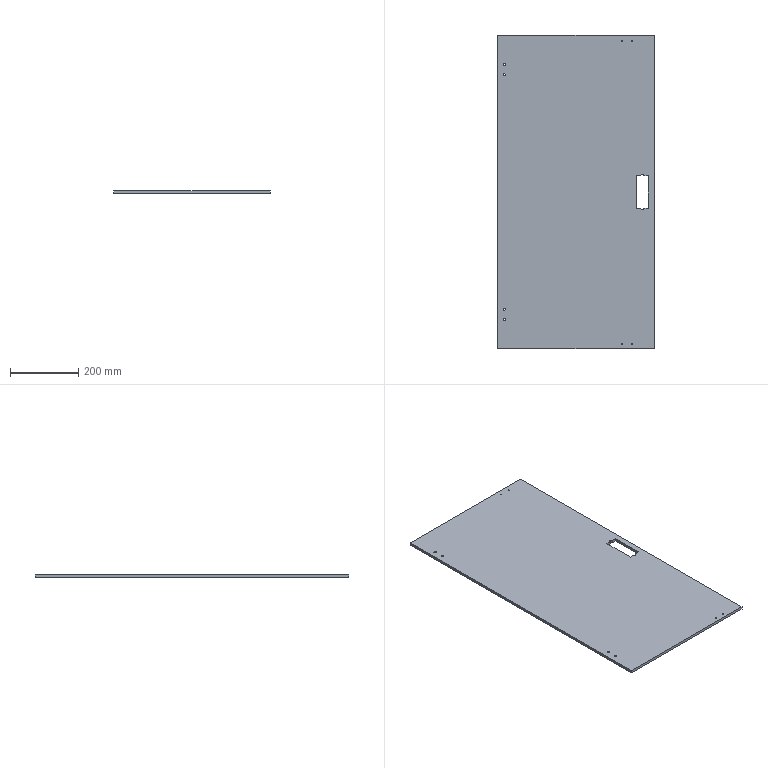Part | STEP file | Left door panel_PN_0002 | 1 solid | 30 faces | box 458.5 x 917 x 8 mm | volume 3334170 mm3 | cylinder 18 | plane 12 | commonest cylinder face diameters 3.3 x8 6.5 x8 8 x2
STEP:
#1=CARTESIAN_POINT('',(-207.,373.5,-4.));
#2=VERTEX_POINT('',#1);
#3=CARTESIAN_POINT('',(-213.5,373.5,-4.));
#4=VERTEX_POINT('',#3);
#5=CARTESIAN_POINT('',(-210.25,373.5,-4.));
#6=DIRECTION('',(0.,0.,-1.));
#7=DIRECTION('',(1.,0.,0.));
#8=AXIS2_PLACEMENT_3D('',#5,#6,#7);
#9=CIRCLE('',#8,3.25);
#10=EDGE_CURVE('',#2,#4,#9,.T.);
#11=ORIENTED_EDGE('',*,*,#10,.T.);
#12=CARTESIAN_POINT('',(-213.5,373.5,4.));
#13=VERTEX_POINT('',#12);
#14=CARTESIAN_POINT('',(-213.5,373.5,-4.));
#15=DIRECTION('',(0.,0.,1.));
#16=VECTOR('',#15,1000.);
#17=LINE('',#14,#16);
#18=EDGE_CURVE('',#4,#13,#17,.T.);
#19=ORIENTED_EDGE('',*,*,#18,.T.);
#20=CARTESIAN_POINT('',(-207.,373.5,4.));
#21=VERTEX_POINT('',#20);
#22=CARTESIAN_POINT('',(-210.25,373.5,4.));
#23=DIRECTION('',(0.,0.,-1.));
#24=DIRECTION('',(1.,0.,0.));
#25=AXIS2_PLACEMENT_3D('',#22,#23,#24);
#26=CIRCLE('',#25,3.25);
#27=EDGE_CURVE('',#21,#13,#26,.T.);
#28=ORIENTED_EDGE('',*,*,#27,.F.);
#29=CARTESIAN_POINT('',(-207.,373.5,-4.));
#30=DIRECTION('',(0.,0.,1.));
#31=VECTOR('',#30,1000.);
#32=LINE('',#29,#31);
#33=EDGE_CURVE('',#2,#21,#32,.T.);
#34=ORIENTED_EDGE('',*,*,#33,.F.);
#35=EDGE_LOOP('',(#11,#19,#28,#34));
#36=FACE_OUTER_BOUND('',#35,.T.);
#37=CARTESIAN_POINT('',(-210.25,373.5,-4.));
#38=DIRECTION('',(0.,0.,1.));
#39=DIRECTION('',(1.,0.,0.));
#40=AXIS2_PLACEMENT_3D('',#37,#38,#39);
#41=CYLINDRICAL_SURFACE('',#40,3.25);
#42=ADVANCED_FACE('',(#36),#41,.F.);
#43=CARTESIAN_POINT('',(-207.,343.5,-4.));
#44=VERTEX_POINT('',#43);
#45=CARTESIAN_POINT('',(-213.5,343.5,-4.));
#46=VERTEX_POINT('',#45);
#47=CARTESIAN_POINT('',(-210.25,343.5,-4.));
#48=DIRECTION('',(0.,0.,-1.));
#49=DIRECTION('',(1.,0.,0.));
#50=AXIS2_PLACEMENT_3D('',#47,#48,#49);
#51=CIRCLE('',#50,3.25);
#52=EDGE_CURVE('',#44,#46,#51,.T.);
#53=ORIENTED_EDGE('',*,*,#52,.T.);
#54=CARTESIAN_POINT('',(-213.5,343.5,4.));
#55=VERTEX_POINT('',#54);
#56=CARTESIAN_POINT('',(-213.5,343.5,-4.));
#57=DIRECTION('',(0.,0.,1.));
#58=VECTOR('',#57,1000.);
#59=LINE('',#56,#58);
#60=EDGE_CURVE('',#46,#55,#59,.T.);
#61=ORIENTED_EDGE('',*,*,#60,.T.);
#62=CARTESIAN_POINT('',(-207.,343.5,4.));
#63=VERTEX_POINT('',#62);
#64=CARTESIAN_POINT('',(-210.25,343.5,4.));
#65=DIRECTION('',(0.,0.,-1.));
#66=DIRECTION('',(1.,0.,0.));
#67=AXIS2_PLACEMENT_3D('',#64,#65,#66);
#68=CIRCLE('',#67,3.25);
#69=EDGE_CURVE('',#63,#55,#68,.T.);
#70=ORIENTED_EDGE('',*,*,#69,.F.);
#71=CARTESIAN_POINT('',(-207.,343.5,-4.));
#72=DIRECTION('',(0.,0.,1.));
#73=VECTOR('',#72,1000.);
#74=LINE('',#71,#73);
#75=EDGE_CURVE('',#44,#63,#74,.T.);
#76=ORIENTED_EDGE('',*,*,#75,.F.);
#77=EDGE_LOOP('',(#53,#61,#70,#76));
#78=FACE_OUTER_BOUND('',#77,.T.);
#79=CARTESIAN_POINT('',(-210.25,343.5,-4.));
#80=DIRECTION('',(0.,0.,1.));
#81=DIRECTION('',(1.,0.,0.));
#82=AXIS2_PLACEMENT_3D('',#79,#80,#81);
#83=CYLINDRICAL_SURFACE('',#82,3.25);
#84=ADVANCED_FACE('',(#78),#83,.F.);
#85=CARTESIAN_POINT('',(-207.,-343.5,-4.));
#86=VERTEX_POINT('',#85);
#87=CARTESIAN_POINT('',(-213.5,-343.5,-4.));
#88=VERTEX_POINT('',#87);
#89=CARTESIAN_POINT('',(-210.25,-343.5,-4.));
#90=DIRECTION('',(0.,0.,-1.));
#91=DIRECTION('',(1.,0.,0.));
#92=AXIS2_PLACEMENT_3D('',#89,#90,#91);
#93=CIRCLE('',#92,3.25);
#94=EDGE_CURVE('',#86,#88,#93,.T.);
#95=ORIENTED_EDGE('',*,*,#94,.T.);
#96=CARTESIAN_POINT('',(-213.5,-343.5,4.));
#97=VERTEX_POINT('',#96);
#98=CARTESIAN_POINT('',(-213.5,-343.5,-4.));
#99=DIRECTION('',(0.,0.,1.));
#100=VECTOR('',#99,1000.);
#101=LINE('',#98,#100);
#102=EDGE_CURVE('',#88,#97,#101,.T.);
#103=ORIENTED_EDGE('',*,*,#102,.T.);
#104=CARTESIAN_POINT('',(-207.,-343.5,4.));
#105=VERTEX_POINT('',#104);
#106=CARTESIAN_POINT('',(-210.25,-343.5,4.));
#107=DIRECTION('',(0.,0.,-1.));
#108=DIRECTION('',(1.,0.,0.));
#109=AXIS2_PLACEMENT_3D('',#106,#107,#108);
#110=CIRCLE('',#109,3.25);
#111=EDGE_CURVE('',#105,#97,#110,.T.);
#112=ORIENTED_EDGE('',*,*,#111,.F.);
#113=CARTESIAN_POINT('',(-207.,-343.5,-4.));
#114=DIRECTION('',(0.,0.,1.));
#115=VECTOR('',#114,1000.);
#116=LINE('',#113,#115);
#117=EDGE_CURVE('',#86,#105,#116,.T.);
#118=ORIENTED_EDGE('',*,*,#117,.F.);
#119=EDGE_LOOP('',(#95,#103,#112,#118));
#120=FACE_OUTER_BOUND('',#119,.T.);
#121=CARTESIAN_POINT('',(-210.25,-343.5,-4.));
#122=DIRECTION('',(0.,0.,1.));
#123=DIRECTION('',(1.,0.,0.));
#124=AXIS2_PLACEMENT_3D('',#121,#122,#123);
#125=CYLINDRICAL_SURFACE('',#124,3.25);
#126=ADVANCED_FACE('',(#120),#125,.F.);
#127=CARTESIAN_POINT('',(-207.,-373.5,-4.));
#128=VERTEX_POINT('',#127);
#129=CARTESIAN_POINT('',(-213.5,-373.5,-4.));
#130=VERTEX_POINT('',#129);
#131=CARTESIAN_POINT('',(-210.25,-373.5,-4.));
#132=DIRECTION('',(0.,0.,-1.));
#133=DIRECTION('',(1.,0.,0.));
#134=AXIS2_PLACEMENT_3D('',#131,#132,#133);
#135=CIRCLE('',#134,3.25);
#136=EDGE_CURVE('',#128,#130,#135,.T.);
#137=ORIENTED_EDGE('',*,*,#136,.T.);
#138=CARTESIAN_POINT('',(-213.5,-373.5,4.));
#139=VERTEX_POINT('',#138);
#140=CARTESIAN_POINT('',(-213.5,-373.5,-4.));
#141=DIRECTION('',(0.,0.,1.));
#142=VECTOR('',#141,1000.);
#143=LINE('',#140,#142);
#144=EDGE_CURVE('',#130,#139,#143,.T.);
#145=ORIENTED_EDGE('',*,*,#144,.T.);
#146=CARTESIAN_POINT('',(-207.,-373.5,4.));
#147=VERTEX_POINT('',#146);
#148=CARTESIAN_POINT('',(-210.25,-373.5,4.));
#149=DIRECTION('',(0.,0.,-1.));
#150=DIRECTION('',(1.,0.,0.));
#151=AXIS2_PLACEMENT_3D('',#148,#149,#150);
#152=CIRCLE('',#151,3.25);
#153=EDGE_CURVE('',#147,#139,#152,.T.);
#154=ORIENTED_EDGE('',*,*,#153,.F.);
#155=CARTESIAN_POINT('',(-207.,-373.5,-4.));
#156=DIRECTION('',(0.,0.,1.));
#157=VECTOR('',#156,1000.);
#158=LINE('',#155,#157);
#159=EDGE_CURVE('',#128,#147,#158,.T.);
#160=ORIENTED_EDGE('',*,*,#159,.F.);
#161=EDGE_LOOP('',(#137,#145,#154,#160));
#162=FACE_OUTER_BOUND('',#161,.T.);
#163=CARTESIAN_POINT('',(-210.25,-373.5,-4.));
#164=DIRECTION('',(0.,0.,1.));
#165=DIRECTION('',(1.,0.,0.));
#166=AXIS2_PLACEMENT_3D('',#163,#164,#165);
#167=CYLINDRICAL_SURFACE('',#166,3.25);
#168=ADVANCED_FACE('',(#162),#167,.F.);
#169=CARTESIAN_POINT('',(135.9,-444.5,4.));
#170=VERTEX_POINT('',#169);
#171=CARTESIAN_POINT('',(132.6,-444.5,4.));
#172=VERTEX_POINT('',#171);
#173=CARTESIAN_POINT('',(134.25,-444.5,4.));
#174=DIRECTION('',(0.,0.,-1.));
#175=DIRECTION('',(-1.,0.,0.));
#176=AXIS2_PLACEMENT_3D('',#173,#174,#175);
#177=CIRCLE('',#176,1.65);
#178=EDGE_CURVE('',#170,#172,#177,.T.);
#179=ORIENTED_EDGE('',*,*,#178,.F.);
#180=CARTESIAN_POINT('',(135.9,-444.5,-4.));
#181=VERTEX_POINT('',#180);
#182=CARTESIAN_POINT('',(135.9,-444.5,-4.));
#183=DIRECTION('',(0.,0.,-1.));
#184=VECTOR('',#183,1000.);
#185=LINE('',#182,#184);
#186=EDGE_CURVE('',#170,#181,#185,.T.);
#187=ORIENTED_EDGE('',*,*,#186,.T.);
#188=CARTESIAN_POINT('',(132.6,-444.5,-4.));
#189=VERTEX_POINT('',#188);
#190=CARTESIAN_POINT('',(134.25,-444.5,-4.));
#191=DIRECTION('',(0.,0.,-1.));
#192=DIRECTION('',(-1.,0.,0.));
#193=AXIS2_PLACEMENT_3D('',#190,#191,#192);
#194=CIRCLE('',#193,1.65);
#195=EDGE_CURVE('',#181,#189,#194,.T.);
#196=ORIENTED_EDGE('',*,*,#195,.T.);
#197=CARTESIAN_POINT('',(132.6,-444.5,-4.));
#198=DIRECTION('',(0.,0.,-1.));
#199=VECTOR('',#198,1000.);
#200=LINE('',#197,#199);
#201=EDGE_CURVE('',#172,#189,#200,.T.);
#202=ORIENTED_EDGE('',*,*,#201,.F.);
#203=EDGE_LOOP('',(#179,#187,#196,#202));
#204=FACE_OUTER_BOUND('',#203,.T.);
#205=CARTESIAN_POINT('',(134.25,-444.5,-4.));
#206=DIRECTION('',(0.,0.,-1.));
#207=DIRECTION('',(-1.,0.,0.));
#208=AXIS2_PLACEMENT_3D('',#205,#206,#207);
#209=CYLINDRICAL_SURFACE('',#208,1.65);
#210=ADVANCED_FACE('',(#204),#209,.F.);
#211=CARTESIAN_POINT('',(165.9,-444.5,4.));
#212=VERTEX_POINT('',#211);
#213=CARTESIAN_POINT('',(162.6,-444.5,4.));
#214=VERTEX_POINT('',#213);
#215=CARTESIAN_POINT('',(164.25,-444.5,4.));
#216=DIRECTION('',(0.,0.,-1.));
#217=DIRECTION('',(-1.,0.,0.));
#218=AXIS2_PLACEMENT_3D('',#215,#216,#217);
#219=CIRCLE('',#218,1.65);
#220=EDGE_CURVE('',#212,#214,#219,.T.);
#221=ORIENTED_EDGE('',*,*,#220,.F.);
#222=CARTESIAN_POINT('',(165.9,-444.5,-4.));
#223=VERTEX_POINT('',#222);
#224=CARTESIAN_POINT('',(165.9,-444.5,-4.));
#225=DIRECTION('',(0.,0.,-1.));
#226=VECTOR('',#225,1000.);
#227=LINE('',#224,#226);
#228=EDGE_CURVE('',#212,#223,#227,.T.);
#229=ORIENTED_EDGE('',*,*,#228,.T.);
#230=CARTESIAN_POINT('',(162.6,-444.5,-4.));
#231=VERTEX_POINT('',#230);
#232=CARTESIAN_POINT('',(164.25,-444.5,-4.));
#233=DIRECTION('',(0.,0.,-1.));
#234=DIRECTION('',(-1.,0.,0.));
#235=AXIS2_PLACEMENT_3D('',#232,#233,#234);
#236=CIRCLE('',#235,1.65);
#237=EDGE_CURVE('',#223,#231,#236,.T.);
#238=ORIENTED_EDGE('',*,*,#237,.T.);
#239=CARTESIAN_POINT('',(162.6,-444.5,-4.));
#240=DIRECTION('',(0.,0.,-1.));
#241=VECTOR('',#240,1000.);
#242=LINE('',#239,#241);
#243=EDGE_CURVE('',#214,#231,#242,.T.);
#244=ORIENTED_EDGE('',*,*,#243,.F.);
#245=EDGE_LOOP('',(#221,#229,#238,#244));
#246=FACE_OUTER_BOUND('',#245,.T.);
#247=CARTESIAN_POINT('',(164.25,-444.5,-4.));
#248=DIRECTION('',(0.,0.,-1.));
#249=DIRECTION('',(-1.,0.,0.));
#250=AXIS2_PLACEMENT_3D('',#247,#248,#249);
#251=CYLINDRICAL_SURFACE('',#250,1.65);
#252=ADVANCED_FACE('',(#246),#251,.F.);
#253=CARTESIAN_POINT('',(135.9,443.5,4.));
#254=VERTEX_POINT('',#253);
#255=CARTESIAN_POINT('',(132.6,443.5,4.));
#256=VERTEX_POINT('',#255);
#257=CARTESIAN_POINT('',(134.25,443.5,4.));
#258=DIRECTION('',(0.,0.,-1.));
#259=DIRECTION('',(-1.,0.,0.));
#260=AXIS2_PLACEMENT_3D('',#257,#258,#259);
#261=CIRCLE('',#260,1.65);
#262=EDGE_CURVE('',#254,#256,#261,.T.);
#263=ORIENTED_EDGE('',*,*,#262,.F.);
#264=CARTESIAN_POINT('',(135.9,443.5,-4.));
#265=VERTEX_POINT('',#264);
#266=CARTESIAN_POINT('',(135.9,443.5,-4.));
#267=DIRECTION('',(0.,0.,-1.));
#268=VECTOR('',#267,1000.);
#269=LINE('',#266,#268);
#270=EDGE_CURVE('',#254,#265,#269,.T.);
#271=ORIENTED_EDGE('',*,*,#270,.T.);
#272=CARTESIAN_POINT('',(132.6,443.5,-4.));
#273=VERTEX_POINT('',#272);
#274=CARTESIAN_POINT('',(134.25,443.5,-4.));
#275=DIRECTION('',(0.,0.,-1.));
#276=DIRECTION('',(-1.,0.,0.));
#277=AXIS2_PLACEMENT_3D('',#274,#275,#276);
#278=CIRCLE('',#277,1.65);
#279=EDGE_CURVE('',#265,#273,#278,.T.);
#280=ORIENTED_EDGE('',*,*,#279,.T.);
#281=CARTESIAN_POINT('',(132.6,443.5,-4.));
#282=DIRECTION('',(0.,0.,-1.));
#283=VECTOR('',#282,1000.);
#284=LINE('',#281,#283);
#285=EDGE_CURVE('',#256,#273,#284,.T.);
#286=ORIENTED_EDGE('',*,*,#285,.F.);
#287=EDGE_LOOP('',(#263,#271,#280,#286));
#288=FACE_OUTER_BOUND('',#287,.T.);
#289=CARTESIAN_POINT('',(134.25,443.5,-4.));
#290=DIRECTION('',(0.,0.,-1.));
#291=DIRECTION('',(-1.,0.,0.));
#292=AXIS2_PLACEMENT_3D('',#289,#290,#291);
#293=CYLINDRICAL_SURFACE('',#292,1.65);
#294=ADVANCED_FACE('',(#288),#293,.F.);
#295=CARTESIAN_POINT('',(165.9,443.5,4.));
#296=VERTEX_POINT('',#295);
#297=CARTESIAN_POINT('',(162.6,443.5,4.));
#298=VERTEX_POINT('',#297);
#299=CARTESIAN_POINT('',(164.25,443.5,4.));
#300=DIRECTION('',(0.,0.,-1.));
#301=DIRECTION('',(-1.,0.,0.));
#302=AXIS2_PLACEMENT_3D('',#299,#300,#301);
#303=CIRCLE('',#302,1.65);
#304=EDGE_CURVE('',#296,#298,#303,.T.);
#305=ORIENTED_EDGE('',*,*,#304,.F.);
#306=CARTESIAN_POINT('',(165.9,443.5,-4.));
#307=VERTEX_POINT('',#306);
#308=CARTESIAN_POINT('',(165.9,443.5,-4.));
#309=DIRECTION('',(0.,0.,-1.));
#310=VECTOR('',#309,1000.);
#311=LINE('',#308,#310);
#312=EDGE_CURVE('',#296,#307,#311,.T.);
#313=ORIENTED_EDGE('',*,*,#312,.T.);
#314=CARTESIAN_POINT('',(162.6,443.5,-4.));
#315=VERTEX_POINT('',#314);
#316=CARTESIAN_POINT('',(164.25,443.5,-4.));
#317=DIRECTION('',(0.,0.,-1.));
#318=DIRECTION('',(-1.,0.,0.));
#319=AXIS2_PLACEMENT_3D('',#316,#317,#318);
#320=CIRCLE('',#319,1.65);
#321=EDGE_CURVE('',#307,#315,#320,.T.);
#322=ORIENTED_EDGE('',*,*,#321,.T.);
#323=CARTESIAN_POINT('',(162.6,443.5,-4.));
#324=DIRECTION('',(0.,0.,-1.));
#325=VECTOR('',#324,1000.);
#326=LINE('',#323,#325);
#327=EDGE_CURVE('',#298,#315,#326,.T.);
#328=ORIENTED_EDGE('',*,*,#327,.F.);
#329=EDGE_LOOP('',(#305,#313,#322,#328));
#330=FACE_OUTER_BOUND('',#329,.T.);
#331=CARTESIAN_POINT('',(164.25,443.5,-4.));
#332=DIRECTION('',(0.,0.,-1.));
#333=DIRECTION('',(-1.,0.,0.));
#334=AXIS2_PLACEMENT_3D('',#331,#332,#333);
#335=CYLINDRICAL_SURFACE('',#334,1.65);
#336=ADVANCED_FACE('',(#330),#335,.F.);
#337=CARTESIAN_POINT('',(190.25,48.,-4.));
#338=VERTEX_POINT('',#337);
#339=CARTESIAN_POINT('',(198.25,48.,-4.));
#340=VERTEX_POINT('',#339);
#341=CARTESIAN_POINT('',(194.25,48.,-4.));
#342=DIRECTION('',(0.,0.,-1.));
#343=DIRECTION('',(1.,0.,0.));
#344=AXIS2_PLACEMENT_3D('',#341,#342,#343);
#345=CIRCLE('',#344,4.);
#346=EDGE_CURVE('',#338,#340,#345,.T.);
#347=ORIENTED_EDGE('',*,*,#346,.F.);
#348=CARTESIAN_POINT('',(176.25,48.,-4.));
#349=VERTEX_POINT('',#348);
#350=CARTESIAN_POINT('',(0.,48.,-4.));
#351=DIRECTION('',(1.,0.,0.));
#352=VECTOR('',#351,1000.);
#353=LINE('',#350,#352);
#354=EDGE_CURVE('',#349,#338,#353,.T.);
#355=ORIENTED_EDGE('',*,*,#354,.F.);
#356=CARTESIAN_POINT('',(176.25,-48.,-4.));
#357=VERTEX_POINT('',#356);
#358=CARTESIAN_POINT('',(176.25,0.,-4.));
#359=DIRECTION('',(0.,1.,0.));
#360=VECTOR('',#359,1000.);
#361=LINE('',#358,#360);
#362=EDGE_CURVE('',#357,#349,#361,.T.);
#363=ORIENTED_EDGE('',*,*,#362,.F.);
#364=CARTESIAN_POINT('',(190.25,-48.,-4.));
#365=VERTEX_POINT('',#364);
#366=CARTESIAN_POINT('',(0.,-48.,-4.));
#367=DIRECTION('',(-1.,0.,0.));
#368=VECTOR('',#367,1000.);
#369=LINE('',#366,#368);
#370=EDGE_CURVE('',#365,#357,#369,.T.);
#371=ORIENTED_EDGE('',*,*,#370,.F.);
#372=CARTESIAN_POINT('',(198.25,-48.,-4.));
#373=VERTEX_POINT('',#372);
#374=CARTESIAN_POINT('',(194.25,-48.,-4.));
#375=DIRECTION('',(0.,0.,-1.));
#376=DIRECTION('',(1.,0.,0.));
#377=AXIS2_PLACEMENT_3D('',#374,#375,#376);
#378=CIRCLE('',#377,4.);
#379=EDGE_CURVE('',#373,#365,#378,.T.);
#380=ORIENTED_EDGE('',*,*,#379,.F.);
#381=CARTESIAN_POINT('',(212.25,-48.,-4.));
#382=VERTEX_POINT('',#381);
#383=CARTESIAN_POINT('',(0.,-48.,-4.));
#384=DIRECTION('',(-1.,0.,0.));
#385=VECTOR('',#384,1000.);
#386=LINE('',#383,#385);
#387=EDGE_CURVE('',#382,#373,#386,.T.);
#388=ORIENTED_EDGE('',*,*,#387,.F.);
#389=CARTESIAN_POINT('',(212.25,48.,-4.));
#390=VERTEX_POINT('',#389);
#391=CARTESIAN_POINT('',(212.25,0.,-4.));
#392=DIRECTION('',(0.,-1.,0.));
#393=VECTOR('',#392,1000.);
#394=LINE('',#391,#393);
#395=EDGE_CURVE('',#390,#382,#394,.T.);
#396=ORIENTED_EDGE('',*,*,#395,.F.);
#397=CARTESIAN_POINT('',(0.,48.,-4.));
#398=DIRECTION('',(1.,0.,0.));
#399=VECTOR('',#398,1000.);
#400=LINE('',#397,#399);
#401=EDGE_CURVE('',#340,#390,#400,.T.);
#402=ORIENTED_EDGE('',*,*,#401,.F.);
#403=EDGE_LOOP('',(#347,#355,#363,#371,#380,#388,#396,#402));
#404=FACE_BOUND('',#403,.T.);
#405=CARTESIAN_POINT('',(-229.25,-458.5,-4.));
#406=VERTEX_POINT('',#405);
#407=CARTESIAN_POINT('',(229.25,-458.5,-4.));
#408=VERTEX_POINT('',#407);
#409=CARTESIAN_POINT('',(0.,-458.5,-4.));
#410=DIRECTION('',(1.,0.,0.));
#411=VECTOR('',#410,1000.);
#412=LINE('',#409,#411);
#413=EDGE_CURVE('',#406,#408,#412,.T.);
#414=ORIENTED_EDGE('',*,*,#413,.F.);
#415=CARTESIAN_POINT('',(-229.25,458.5,-4.));
#416=VERTEX_POINT('',#415);
#417=CARTESIAN_POINT('',(-229.25,0.,-4.));
#418=DIRECTION('',(0.,-1.,0.));
#419=VECTOR('',#418,1000.);
#420=LINE('',#417,#419);
#421=EDGE_CURVE('',#416,#406,#420,.T.);
#422=ORIENTED_EDGE('',*,*,#421,.F.);
#423=CARTESIAN_POINT('',(229.25,458.5,-4.));
#424=VERTEX_POINT('',#423);
#425=CARTESIAN_POINT('',(0.,458.5,-4.));
#426=DIRECTION('',(-1.,0.,0.));
#427=VECTOR('',#426,1000.);
#428=LINE('',#425,#427);
#429=EDGE_CURVE('',#424,#416,#428,.T.);
#430=ORIENTED_EDGE('',*,*,#429,.F.);
#431=CARTESIAN_POINT('',(229.25,0.,-4.));
#432=DIRECTION('',(0.,1.,0.));
#433=VECTOR('',#432,1000.);
#434=LINE('',#431,#433);
#435=EDGE_CURVE('',#408,#424,#434,.T.);
#436=ORIENTED_EDGE('',*,*,#435,.F.);
#437=EDGE_LOOP('',(#414,#422,#430,#436));
#438=FACE_OUTER_BOUND('',#437,.T.);
#439=ORIENTED_EDGE('',*,*,#10,.F.);
#440=CARTESIAN_POINT('',(-210.25,373.5,-4.));
#441=DIRECTION('',(0.,0.,-1.));
#442=DIRECTION('',(1.,0.,0.));
#443=AXIS2_PLACEMENT_3D('',#440,#441,#442);
#444=CIRCLE('',#443,3.25);
#445=EDGE_CURVE('',#4,#2,#444,.T.);
#446=ORIENTED_EDGE('',*,*,#445,.F.);
#447=EDGE_LOOP('',(#439,#446));
#448=FACE_BOUND('',#447,.T.);
#449=ORIENTED_EDGE('',*,*,#52,.F.);
#450=CARTESIAN_POINT('',(-210.25,343.5,-4.));
#451=DIRECTION('',(0.,0.,-1.));
#452=DIRECTION('',(1.,0.,0.));
#453=AXIS2_PLACEMENT_3D('',#450,#451,#452);
#454=CIRCLE('',#453,3.25);
#455=EDGE_CURVE('',#46,#44,#454,.T.);
#456=ORIENTED_EDGE('',*,*,#455,.F.);
#457=EDGE_LOOP('',(#449,#456));
#458=FACE_BOUND('',#457,.T.);
#459=ORIENTED_EDGE('',*,*,#94,.F.);
#460=CARTESIAN_POINT('',(-210.25,-343.5,-4.));
#461=DIRECTION('',(0.,0.,-1.));
#462=DIRECTION('',(1.,0.,0.));
#463=AXIS2_PLACEMENT_3D('',#460,#461,#462);
#464=CIRCLE('',#463,3.25);
#465=EDGE_CURVE('',#88,#86,#464,.T.);
#466=ORIENTED_EDGE('',*,*,#465,.F.);
#467=EDGE_LOOP('',(#459,#466));
#468=FACE_BOUND('',#467,.T.);
#469=ORIENTED_EDGE('',*,*,#136,.F.);
#470=CARTESIAN_POINT('',(-210.25,-373.5,-4.));
#471=DIRECTION('',(0.,0.,-1.));
#472=DIRECTION('',(1.,0.,0.));
#473=AXIS2_PLACEMENT_3D('',#470,#471,#472);
#474=CIRCLE('',#473,3.25);
#475=EDGE_CURVE('',#130,#128,#474,.T.);
#476=ORIENTED_EDGE('',*,*,#475,.F.);
#477=EDGE_LOOP('',(#469,#476));
#478=FACE_BOUND('',#477,.T.);
#479=CARTESIAN_POINT('',(134.25,-444.5,-4.));
#480=DIRECTION('',(0.,0.,-1.));
#481=DIRECTION('',(-1.,0.,0.));
#482=AXIS2_PLACEMENT_3D('',#479,#480,#481);
#483=CIRCLE('',#482,1.65);
#484=EDGE_CURVE('',#189,#181,#483,.T.);
#485=ORIENTED_EDGE('',*,*,#484,.F.);
#486=ORIENTED_EDGE('',*,*,#195,.F.);
#487=EDGE_LOOP('',(#485,#486));
#488=FACE_BOUND('',#487,.T.);
#489=CARTESIAN_POINT('',(164.25,-444.5,-4.));
#490=DIRECTION('',(0.,0.,-1.));
#491=DIRECTION('',(-1.,0.,0.));
#492=AXIS2_PLACEMENT_3D('',#489,#490,#491);
#493=CIRCLE('',#492,1.65);
#494=EDGE_CURVE('',#231,#223,#493,.T.);
#495=ORIENTED_EDGE('',*,*,#494,.F.);
#496=ORIENTED_EDGE('',*,*,#237,.F.);
#497=EDGE_LOOP('',(#495,#496));
#498=FACE_BOUND('',#497,.T.);
#499=CARTESIAN_POINT('',(134.25,443.5,-4.));
#500=DIRECTION('',(0.,0.,-1.));
#501=DIRECTION('',(-1.,0.,0.));
#502=AXIS2_PLACEMENT_3D('',#499,#500,#501);
#503=CIRCLE('',#502,1.65);
#504=EDGE_CURVE('',#273,#265,#503,.T.);
#505=ORIENTED_EDGE('',*,*,#504,.F.);
#506=ORIENTED_EDGE('',*,*,#279,.F.);
#507=EDGE_LOOP('',(#505,#506));
#508=FACE_BOUND('',#507,.T.);
#509=CARTESIAN_POINT('',(164.25,443.5,-4.));
#510=DIRECTION('',(0.,0.,-1.));
#511=DIRECTION('',(-1.,0.,0.));
#512=AXIS2_PLACEMENT_3D('',#509,#510,#511);
#513=CIRCLE('',#512,1.65);
#514=EDGE_CURVE('',#315,#307,#513,.T.);
#515=ORIENTED_EDGE('',*,*,#514,.F.);
#516=ORIENTED_EDGE('',*,*,#321,.F.);
#517=EDGE_LOOP('',(#515,#516));
#518=FACE_BOUND('',#517,.T.);
#519=CARTESIAN_POINT('',(0.,0.,-4.));
#520=DIRECTION('',(0.,0.,1.));
#521=DIRECTION('',(1.,0.,0.));
#522=AXIS2_PLACEMENT_3D('',#519,#520,#521);
#523=PLANE('',#522);
#524=ADVANCED_FACE('',(#404,#438,#448,#458,#468,#478,#488,#498,#508,#518),#523,.F.);
#525=ORIENTED_EDGE('',*,*,#401,.T.);
#526=CARTESIAN_POINT('',(212.25,48.,4.));
#527=VERTEX_POINT('',#526);
#528=CARTESIAN_POINT('',(212.25,48.,-4.));
#529=DIRECTION('',(0.,0.,1.));
#530=VECTOR('',#529,1000.);
#531=LINE('',#528,#530);
#532=EDGE_CURVE('',#390,#527,#531,.T.);
#533=ORIENTED_EDGE('',*,*,#532,.T.);
#534=CARTESIAN_POINT('',(198.25,48.,4.));
#535=VERTEX_POINT('',#534);
#536=CARTESIAN_POINT('',(0.,48.,4.));
#537=DIRECTION('',(-1.,0.,0.));
#538=VECTOR('',#537,1000.);
#539=LINE('',#536,#538);
#540=EDGE_CURVE('',#527,#535,#539,.T.);
#541=ORIENTED_EDGE('',*,*,#540,.T.);
#542=CARTESIAN_POINT('',(198.25,48.,-4.));
#543=DIRECTION('',(0.,0.,-1.));
#544=VECTOR('',#543,1000.);
#545=LINE('',#542,#544);
#546=EDGE_CURVE('',#535,#340,#545,.T.);
#547=ORIENTED_EDGE('',*,*,#546,.T.);
#548=EDGE_LOOP('',(#525,#533,#541,#547));
#549=FACE_OUTER_BOUND('',#548,.T.);
#550=CARTESIAN_POINT('',(0.,48.,-4.));
#551=DIRECTION('',(0.,-1.,0.));
#552=DIRECTION('',(1.,0.,0.));
#553=AXIS2_PLACEMENT_3D('',#550,#551,#552);
#554=PLANE('',#553);
#555=ADVANCED_FACE('',(#549),#554,.T.);
#556=CARTESIAN_POINT('',(190.25,48.,4.));
#557=VERTEX_POINT('',#556);
#558=CARTESIAN_POINT('',(190.25,48.,-4.));
#559=DIRECTION('',(0.,0.,1.));
#560=VECTOR('',#559,1000.);
#561=LINE('',#558,#560);
#562=EDGE_CURVE('',#338,#557,#561,.T.);
#563=ORIENTED_EDGE('',*,*,#562,.F.);
#564=ORIENTED_EDGE('',*,*,#346,.T.);
#565=ORIENTED_EDGE('',*,*,#546,.F.);
#566=CARTESIAN_POINT('',(194.25,48.,4.));
#567=DIRECTION('',(0.,0.,-1.));
#568=DIRECTION('',(1.,0.,0.));
#569=AXIS2_PLACEMENT_3D('',#566,#567,#568);
#570=CIRCLE('',#569,4.);
#571=EDGE_CURVE('',#557,#535,#570,.T.);
#572=ORIENTED_EDGE('',*,*,#571,.F.);
#573=EDGE_LOOP('',(#563,#564,#565,#572));
#574=FACE_OUTER_BOUND('',#573,.T.);
#575=CARTESIAN_POINT('',(194.25,48.,-4.));
#576=DIRECTION('',(0.,0.,1.));
#577=DIRECTION('',(1.,0.,0.));
#578=AXIS2_PLACEMENT_3D('',#575,#576,#577);
#579=CYLINDRICAL_SURFACE('',#578,4.);
#580=ADVANCED_FACE('',(#574),#579,.F.);
#581=ORIENTED_EDGE('',*,*,#354,.T.);
#582=ORIENTED_EDGE('',*,*,#562,.T.);
#583=CARTESIAN_POINT('',(176.25,48.,4.));
#584=VERTEX_POINT('',#583);
#585=CARTESIAN_POINT('',(0.,48.,4.));
#586=DIRECTION('',(-1.,0.,0.));
#587=VECTOR('',#586,1000.);
#588=LINE('',#585,#587);
#589=EDGE_CURVE('',#557,#584,#588,.T.);
#590=ORIENTED_EDGE('',*,*,#589,.T.);
#591=CARTESIAN_POINT('',(176.25,48.,-4.));
#592=DIRECTION('',(0.,0.,-1.));
#593=VECTOR('',#592,1000.);
#594=LINE('',#591,#593);
#595=EDGE_CURVE('',#584,#349,#594,.T.);
#596=ORIENTED_EDGE('',*,*,#595,.T.);
#597=EDGE_LOOP('',(#581,#582,#590,#596));
#598=FACE_OUTER_BOUND('',#597,.T.);
#599=CARTESIAN_POINT('',(0.,48.,-4.));
#600=DIRECTION('',(0.,-1.,0.));
#601=DIRECTION('',(1.,0.,0.));
#602=AXIS2_PLACEMENT_3D('',#599,#600,#601);
#603=PLANE('',#602);
#604=ADVANCED_FACE('',(#598),#603,.T.);
#605=CARTESIAN_POINT('',(176.25,-48.,4.));
#606=VERTEX_POINT('',#605);
#607=CARTESIAN_POINT('',(176.25,-48.,-4.));
#608=DIRECTION('',(0.,0.,1.));
#609=VECTOR('',#608,1000.);
#610=LINE('',#607,#609);
#611=EDGE_CURVE('',#357,#606,#610,.T.);
#612=ORIENTED_EDGE('',*,*,#611,.F.);
#613=ORIENTED_EDGE('',*,*,#362,.T.);
#614=ORIENTED_EDGE('',*,*,#595,.F.);
#615=CARTESIAN_POINT('',(176.25,0.,4.));
#616=DIRECTION('',(0.,1.,0.));
#617=VECTOR('',#616,1000.);
#618=LINE('',#615,#617);
#619=EDGE_CURVE('',#606,#584,#618,.T.);
#620=ORIENTED_EDGE('',*,*,#619,.F.);
#621=EDGE_LOOP('',(#612,#613,#614,#620));
#622=FACE_OUTER_BOUND('',#621,.T.);
#623=CARTESIAN_POINT('',(176.25,0.,-4.));
#624=DIRECTION('',(-1.,0.,0.));
#625=DIRECTION('',(0.,-1.,0.));
#626=AXIS2_PLACEMENT_3D('',#623,#624,#625);
#627=PLANE('',#626);
#628=ADVANCED_FACE('',(#622),#627,.F.);
#629=CARTESIAN_POINT('',(190.25,-48.,4.));
#630=VERTEX_POINT('',#629);
#631=CARTESIAN_POINT('',(190.25,-48.,-4.));
#632=DIRECTION('',(0.,0.,1.));
#633=VECTOR('',#632,1000.);
#634=LINE('',#631,#633);
#635=EDGE_CURVE('',#365,#630,#634,.T.);
#636=ORIENTED_EDGE('',*,*,#635,.F.);
#637=ORIENTED_EDGE('',*,*,#370,.T.);
#638=ORIENTED_EDGE('',*,*,#611,.T.);
#639=CARTESIAN_POINT('',(0.,-48.,4.));
#640=DIRECTION('',(-1.,0.,0.));
#641=VECTOR('',#640,1000.);
#642=LINE('',#639,#641);
#643=EDGE_CURVE('',#630,#606,#642,.T.);
#644=ORIENTED_EDGE('',*,*,#643,.F.);
#645=EDGE_LOOP('',(#636,#637,#638,#644));
#646=FACE_OUTER_BOUND('',#645,.T.);
#647=CARTESIAN_POINT('',(0.,-48.,-4.));
#648=DIRECTION('',(0.,-1.,0.));
#649=DIRECTION('',(0.,0.,-1.));
#650=AXIS2_PLACEMENT_3D('',#647,#648,#649);
#651=PLANE('',#650);
#652=ADVANCED_FACE('',(#646),#651,.F.);
#653=CARTESIAN_POINT('',(198.25,-48.,4.));
#654=VERTEX_POINT('',#653);
#655=CARTESIAN_POINT('',(198.25,-48.,-4.));
#656=DIRECTION('',(0.,0.,1.));
#657=VECTOR('',#656,1000.);
#658=LINE('',#655,#657);
#659=EDGE_CURVE('',#373,#654,#658,.T.);
#660=ORIENTED_EDGE('',*,*,#659,.F.);
#661=ORIENTED_EDGE('',*,*,#379,.T.);
#662=ORIENTED_EDGE('',*,*,#635,.T.);
#663=CARTESIAN_POINT('',(194.25,-48.,4.));
#664=DIRECTION('',(0.,0.,-1.));
#665=DIRECTION('',(1.,0.,0.));
#666=AXIS2_PLACEMENT_3D('',#663,#664,#665);
#667=CIRCLE('',#666,4.);
#668=EDGE_CURVE('',#654,#630,#667,.T.);
#669=ORIENTED_EDGE('',*,*,#668,.F.);
#670=EDGE_LOOP('',(#660,#661,#662,#669));
#671=FACE_OUTER_BOUND('',#670,.T.);
#672=CARTESIAN_POINT('',(194.25,-48.,-4.));
#673=DIRECTION('',(0.,0.,1.));
#674=DIRECTION('',(1.,0.,0.));
#675=AXIS2_PLACEMENT_3D('',#672,#673,#674);
#676=CYLINDRICAL_SURFACE('',#675,4.);
#677=ADVANCED_FACE('',(#671),#676,.F.);
#678=CARTESIAN_POINT('',(212.25,-48.,4.));
#679=VERTEX_POINT('',#678);
#680=CARTESIAN_POINT('',(212.25,-48.,-4.));
#681=DIRECTION('',(0.,0.,1.));
#682=VECTOR('',#681,1000.);
#683=LINE('',#680,#682);
#684=EDGE_CURVE('',#382,#679,#683,.T.);
#685=ORIENTED_EDGE('',*,*,#684,.F.);
#686=ORIENTED_EDGE('',*,*,#387,.T.);
#687=ORIENTED_EDGE('',*,*,#659,.T.);
#688=CARTESIAN_POINT('',(0.,-48.,4.));
#689=DIRECTION('',(-1.,0.,0.));
#690=VECTOR('',#689,1000.);
#691=LINE('',#688,#690);
#692=EDGE_CURVE('',#679,#654,#691,.T.);
#693=ORIENTED_EDGE('',*,*,#692,.F.);
#694=EDGE_LOOP('',(#685,#686,#687,#693));
#695=FACE_OUTER_BOUND('',#694,.T.);
#696=CARTESIAN_POINT('',(0.,-48.,-4.));
#697=DIRECTION('',(0.,-1.,0.));
#698=DIRECTION('',(0.,0.,-1.));
#699=AXIS2_PLACEMENT_3D('',#696,#697,#698);
#700=PLANE('',#699);
#701=ADVANCED_FACE('',(#695),#700,.F.);
#702=ORIENTED_EDGE('',*,*,#395,.T.);
#703=ORIENTED_EDGE('',*,*,#684,.T.);
#704=CARTESIAN_POINT('',(212.25,0.,4.));
#705=DIRECTION('',(0.,1.,0.));
#706=VECTOR('',#705,1000.);
#707=LINE('',#704,#706);
#708=EDGE_CURVE('',#679,#527,#707,.T.);
#709=ORIENTED_EDGE('',*,*,#708,.T.);
#710=ORIENTED_EDGE('',*,*,#532,.F.);
#711=EDGE_LOOP('',(#702,#703,#709,#710));
#712=FACE_OUTER_BOUND('',#711,.T.);
#713=CARTESIAN_POINT('',(212.25,0.,-4.));
#714=DIRECTION('',(-1.,0.,0.));
#715=DIRECTION('',(0.,-1.,0.));
#716=AXIS2_PLACEMENT_3D('',#713,#714,#715);
#717=PLANE('',#716);
#718=ADVANCED_FACE('',(#712),#717,.T.);
#719=CARTESIAN_POINT('',(229.25,458.5,4.));
#720=VERTEX_POINT('',#719);
#721=CARTESIAN_POINT('',(229.25,458.5,4.));
#722=DIRECTION('',(0.,0.,-1.));
#723=VECTOR('',#722,1000.);
#724=LINE('',#721,#723);
#725=EDGE_CURVE('',#720,#424,#724,.T.);
#726=ORIENTED_EDGE('',*,*,#725,.F.);
#727=CARTESIAN_POINT('',(229.25,-458.5,4.));
#728=VERTEX_POINT('',#727);
#729=CARTESIAN_POINT('',(229.25,458.5,4.));
#730=DIRECTION('',(0.,1.,0.));
#731=VECTOR('',#730,1000.);
#732=LINE('',#729,#731);
#733=EDGE_CURVE('',#728,#720,#732,.T.);
#734=ORIENTED_EDGE('',*,*,#733,.F.);
#735=CARTESIAN_POINT('',(229.25,-458.5,4.));
#736=DIRECTION('',(0.,0.,1.));
#737=VECTOR('',#736,1000.);
#738=LINE('',#735,#737);
#739=EDGE_CURVE('',#408,#728,#738,.T.);
#740=ORIENTED_EDGE('',*,*,#739,.F.);
#741=ORIENTED_EDGE('',*,*,#435,.T.);
#742=EDGE_LOOP('',(#726,#734,#740,#741));
#743=FACE_OUTER_BOUND('',#742,.T.);
#744=CARTESIAN_POINT('',(229.25,458.5,4.));
#745=DIRECTION('',(-1.,0.,0.));
#746=DIRECTION('',(0.,-1.,0.));
#747=AXIS2_PLACEMENT_3D('',#744,#745,#746);
#748=PLANE('',#747);
#749=ADVANCED_FACE('',(#743),#748,.F.);
#750=ORIENTED_EDGE('',*,*,#739,.T.);
#751=CARTESIAN_POINT('',(-229.25,-458.5,4.));
#752=VERTEX_POINT('',#751);
#753=CARTESIAN_POINT('',(-229.25,-458.5,4.));
#754=DIRECTION('',(1.,0.,0.));
#755=VECTOR('',#754,1000.);
#756=LINE('',#753,#755);
#757=EDGE_CURVE('',#752,#728,#756,.T.);
#758=ORIENTED_EDGE('',*,*,#757,.F.);
#759=CARTESIAN_POINT('',(-229.25,-458.5,4.));
#760=DIRECTION('',(0.,0.,1.));
#761=VECTOR('',#760,1000.);
#762=LINE('',#759,#761);
#763=EDGE_CURVE('',#406,#752,#762,.T.);
#764=ORIENTED_EDGE('',*,*,#763,.F.);
#765=ORIENTED_EDGE('',*,*,#413,.T.);
#766=EDGE_LOOP('',(#750,#758,#764,#765));
#767=FACE_OUTER_BOUND('',#766,.T.);
#768=CARTESIAN_POINT('',(-229.25,-458.5,4.));
#769=DIRECTION('',(0.,1.,0.));
#770=DIRECTION('',(0.,0.,1.));
#771=AXIS2_PLACEMENT_3D('',#768,#769,#770);
#772=PLANE('',#771);
#773=ADVANCED_FACE('',(#767),#772,.F.);
#774=ORIENTED_EDGE('',*,*,#763,.T.);
#775=CARTESIAN_POINT('',(-229.25,458.5,4.));
#776=VERTEX_POINT('',#775);
#777=CARTESIAN_POINT('',(-229.25,458.5,4.));
#778=DIRECTION('',(0.,-1.,0.));
#779=VECTOR('',#778,1000.);
#780=LINE('',#777,#779);
#781=EDGE_CURVE('',#776,#752,#780,.T.);
#782=ORIENTED_EDGE('',*,*,#781,.F.);
#783=CARTESIAN_POINT('',(-229.25,458.5,4.));
#784=DIRECTION('',(0.,0.,1.));
#785=VECTOR('',#784,1000.);
#786=LINE('',#783,#785);
#787=EDGE_CURVE('',#416,#776,#786,.T.);
#788=ORIENTED_EDGE('',*,*,#787,.F.);
#789=ORIENTED_EDGE('',*,*,#421,.T.);
#790=EDGE_LOOP('',(#774,#782,#788,#789));
#791=FACE_OUTER_BOUND('',#790,.T.);
#792=CARTESIAN_POINT('',(-229.25,458.5,4.));
#793=DIRECTION('',(1.,0.,0.));
#794=DIRECTION('',(0.,1.,0.));
#795=AXIS2_PLACEMENT_3D('',#792,#793,#794);
#796=PLANE('',#795);
#797=ADVANCED_FACE('',(#791),#796,.F.);
#798=ORIENTED_EDGE('',*,*,#787,.T.);
#799=CARTESIAN_POINT('',(-229.25,458.5,4.));
#800=DIRECTION('',(-1.,0.,0.));
#801=VECTOR('',#800,1000.);
#802=LINE('',#799,#801);
#803=EDGE_CURVE('',#720,#776,#802,.T.);
#804=ORIENTED_EDGE('',*,*,#803,.F.);
#805=ORIENTED_EDGE('',*,*,#725,.T.);
#806=ORIENTED_EDGE('',*,*,#429,.T.);
#807=EDGE_LOOP('',(#798,#804,#805,#806));
#808=FACE_OUTER_BOUND('',#807,.T.);
#809=CARTESIAN_POINT('',(-229.25,458.5,4.));
#810=DIRECTION('',(0.,-1.,0.));
#811=DIRECTION('',(0.,0.,-1.));
#812=AXIS2_PLACEMENT_3D('',#809,#810,#811);
#813=PLANE('',#812);
#814=ADVANCED_FACE('',(#808),#813,.F.);
#815=ORIENTED_EDGE('',*,*,#18,.F.);
#816=ORIENTED_EDGE('',*,*,#445,.T.);
#817=ORIENTED_EDGE('',*,*,#33,.T.);
#818=CARTESIAN_POINT('',(-210.25,373.5,4.));
#819=DIRECTION('',(0.,0.,-1.));
#820=DIRECTION('',(1.,0.,0.));
#821=AXIS2_PLACEMENT_3D('',#818,#819,#820);
#822=CIRCLE('',#821,3.25);
#823=EDGE_CURVE('',#13,#21,#822,.T.);
#824=ORIENTED_EDGE('',*,*,#823,.F.);
#825=EDGE_LOOP('',(#815,#816,#817,#824));
#826=FACE_OUTER_BOUND('',#825,.T.);
#827=CARTESIAN_POINT('',(-210.25,373.5,-4.));
#828=DIRECTION('',(0.,0.,1.));
#829=DIRECTION('',(1.,0.,0.));
#830=AXIS2_PLACEMENT_3D('',#827,#828,#829);
#831=CYLINDRICAL_SURFACE('',#830,3.25);
#832=ADVANCED_FACE('',(#826),#831,.F.);
#833=ORIENTED_EDGE('',*,*,#60,.F.);
#834=ORIENTED_EDGE('',*,*,#455,.T.);
#835=ORIENTED_EDGE('',*,*,#75,.T.);
#836=CARTESIAN_POINT('',(-210.25,343.5,4.));
#837=DIRECTION('',(0.,0.,-1.));
#838=DIRECTION('',(1.,0.,0.));
#839=AXIS2_PLACEMENT_3D('',#836,#837,#838);
#840=CIRCLE('',#839,3.25);
#841=EDGE_CURVE('',#55,#63,#840,.T.);
#842=ORIENTED_EDGE('',*,*,#841,.F.);
#843=EDGE_LOOP('',(#833,#834,#835,#842));
#844=FACE_OUTER_BOUND('',#843,.T.);
#845=CARTESIAN_POINT('',(-210.25,343.5,-4.));
#846=DIRECTION('',(0.,0.,1.));
#847=DIRECTION('',(1.,0.,0.));
#848=AXIS2_PLACEMENT_3D('',#845,#846,#847);
#849=CYLINDRICAL_SURFACE('',#848,3.25);
#850=ADVANCED_FACE('',(#844),#849,.F.);
#851=ORIENTED_EDGE('',*,*,#102,.F.);
#852=ORIENTED_EDGE('',*,*,#465,.T.);
#853=ORIENTED_EDGE('',*,*,#117,.T.);
#854=CARTESIAN_POINT('',(-210.25,-343.5,4.));
#855=DIRECTION('',(0.,0.,-1.));
#856=DIRECTION('',(1.,0.,0.));
#857=AXIS2_PLACEMENT_3D('',#854,#855,#856);
#858=CIRCLE('',#857,3.25);
#859=EDGE_CURVE('',#97,#105,#858,.T.);
#860=ORIENTED_EDGE('',*,*,#859,.F.);
#861=EDGE_LOOP('',(#851,#852,#853,#860));
#862=FACE_OUTER_BOUND('',#861,.T.);
#863=CARTESIAN_POINT('',(-210.25,-343.5,-4.));
#864=DIRECTION('',(0.,0.,1.));
#865=DIRECTION('',(1.,0.,0.));
#866=AXIS2_PLACEMENT_3D('',#863,#864,#865);
#867=CYLINDRICAL_SURFACE('',#866,3.25);
#868=ADVANCED_FACE('',(#862),#867,.F.);
#869=ORIENTED_EDGE('',*,*,#144,.F.);
#870=ORIENTED_EDGE('',*,*,#475,.T.);
#871=ORIENTED_EDGE('',*,*,#159,.T.);
#872=CARTESIAN_POINT('',(-210.25,-373.5,4.));
#873=DIRECTION('',(0.,0.,-1.));
#874=DIRECTION('',(1.,0.,0.));
#875=AXIS2_PLACEMENT_3D('',#872,#873,#874);
#876=CIRCLE('',#875,3.25);
#877=EDGE_CURVE('',#139,#147,#876,.T.);
#878=ORIENTED_EDGE('',*,*,#877,.F.);
#879=EDGE_LOOP('',(#869,#870,#871,#878));
#880=FACE_OUTER_BOUND('',#879,.T.);
#881=CARTESIAN_POINT('',(-210.25,-373.5,-4.));
#882=DIRECTION('',(0.,0.,1.));
#883=DIRECTION('',(1.,0.,0.));
#884=AXIS2_PLACEMENT_3D('',#881,#882,#883);
#885=CYLINDRICAL_SURFACE('',#884,3.25);
#886=ADVANCED_FACE('',(#880),#885,.F.);
#887=ORIENTED_EDGE('',*,*,#186,.F.);
#888=CARTESIAN_POINT('',(134.25,-444.5,4.));
#889=DIRECTION('',(0.,0.,-1.));
#890=DIRECTION('',(-1.,0.,0.));
#891=AXIS2_PLACEMENT_3D('',#888,#889,#890);
#892=CIRCLE('',#891,1.65);
#893=EDGE_CURVE('',#172,#170,#892,.T.);
#894=ORIENTED_EDGE('',*,*,#893,.F.);
#895=ORIENTED_EDGE('',*,*,#201,.T.);
#896=ORIENTED_EDGE('',*,*,#484,.T.);
#897=EDGE_LOOP('',(#887,#894,#895,#896));
#898=FACE_OUTER_BOUND('',#897,.T.);
#899=CARTESIAN_POINT('',(134.25,-444.5,-4.));
#900=DIRECTION('',(0.,0.,-1.));
#901=DIRECTION('',(-1.,0.,0.));
#902=AXIS2_PLACEMENT_3D('',#899,#900,#901);
#903=CYLINDRICAL_SURFACE('',#902,1.65);
#904=ADVANCED_FACE('',(#898),#903,.F.);
#905=ORIENTED_EDGE('',*,*,#228,.F.);
#906=CARTESIAN_POINT('',(164.25,-444.5,4.));
#907=DIRECTION('',(0.,0.,-1.));
#908=DIRECTION('',(-1.,0.,0.));
#909=AXIS2_PLACEMENT_3D('',#906,#907,#908);
#910=CIRCLE('',#909,1.65);
#911=EDGE_CURVE('',#214,#212,#910,.T.);
#912=ORIENTED_EDGE('',*,*,#911,.F.);
#913=ORIENTED_EDGE('',*,*,#243,.T.);
#914=ORIENTED_EDGE('',*,*,#494,.T.);
#915=EDGE_LOOP('',(#905,#912,#913,#914));
#916=FACE_OUTER_BOUND('',#915,.T.);
#917=CARTESIAN_POINT('',(164.25,-444.5,-4.));
#918=DIRECTION('',(0.,0.,-1.));
#919=DIRECTION('',(-1.,0.,0.));
#920=AXIS2_PLACEMENT_3D('',#917,#918,#919);
#921=CYLINDRICAL_SURFACE('',#920,1.65);
#922=ADVANCED_FACE('',(#916),#921,.F.);
#923=ORIENTED_EDGE('',*,*,#270,.F.);
#924=CARTESIAN_POINT('',(134.25,443.5,4.));
#925=DIRECTION('',(0.,0.,-1.));
#926=DIRECTION('',(-1.,0.,0.));
#927=AXIS2_PLACEMENT_3D('',#924,#925,#926);
#928=CIRCLE('',#927,1.65);
#929=EDGE_CURVE('',#256,#254,#928,.T.);
#930=ORIENTED_EDGE('',*,*,#929,.F.);
#931=ORIENTED_EDGE('',*,*,#285,.T.);
#932=ORIENTED_EDGE('',*,*,#504,.T.);
#933=EDGE_LOOP('',(#923,#930,#931,#932));
#934=FACE_OUTER_BOUND('',#933,.T.);
#935=CARTESIAN_POINT('',(134.25,443.5,-4.));
#936=DIRECTION('',(0.,0.,-1.));
#937=DIRECTION('',(-1.,0.,0.));
#938=AXIS2_PLACEMENT_3D('',#935,#936,#937);
#939=CYLINDRICAL_SURFACE('',#938,1.65);
#940=ADVANCED_FACE('',(#934),#939,.F.);
#941=ORIENTED_EDGE('',*,*,#312,.F.);
#942=CARTESIAN_POINT('',(164.25,443.5,4.));
#943=DIRECTION('',(0.,0.,-1.));
#944=DIRECTION('',(-1.,0.,0.));
#945=AXIS2_PLACEMENT_3D('',#942,#943,#944);
#946=CIRCLE('',#945,1.65);
#947=EDGE_CURVE('',#298,#296,#946,.T.);
#948=ORIENTED_EDGE('',*,*,#947,.F.);
#949=ORIENTED_EDGE('',*,*,#327,.T.);
#950=ORIENTED_EDGE('',*,*,#514,.T.);
#951=EDGE_LOOP('',(#941,#948,#949,#950));
#952=FACE_OUTER_BOUND('',#951,.T.);
#953=CARTESIAN_POINT('',(164.25,443.5,-4.));
#954=DIRECTION('',(0.,0.,-1.));
#955=DIRECTION('',(-1.,0.,0.));
#956=AXIS2_PLACEMENT_3D('',#953,#954,#955);
#957=CYLINDRICAL_SURFACE('',#956,1.65);
#958=ADVANCED_FACE('',(#952),#957,.F.);
#959=ORIENTED_EDGE('',*,*,#619,.T.);
#960=ORIENTED_EDGE('',*,*,#589,.F.);
#961=ORIENTED_EDGE('',*,*,#571,.T.);
#962=ORIENTED_EDGE('',*,*,#540,.F.);
#963=ORIENTED_EDGE('',*,*,#708,.F.);
#964=ORIENTED_EDGE('',*,*,#692,.T.);
#965=ORIENTED_EDGE('',*,*,#668,.T.);
#966=ORIENTED_EDGE('',*,*,#643,.T.);
#967=EDGE_LOOP('',(#959,#960,#961,#962,#963,#964,#965,#966));
#968=FACE_BOUND('',#967,.T.);
#969=ORIENTED_EDGE('',*,*,#781,.T.);
#970=ORIENTED_EDGE('',*,*,#757,.T.);
#971=ORIENTED_EDGE('',*,*,#733,.T.);
#972=ORIENTED_EDGE('',*,*,#803,.T.);
#973=EDGE_LOOP('',(#969,#970,#971,#972));
#974=FACE_OUTER_BOUND('',#973,.T.);
#975=ORIENTED_EDGE('',*,*,#27,.T.);
#976=ORIENTED_EDGE('',*,*,#823,.T.);
#977=EDGE_LOOP('',(#975,#976));
#978=FACE_BOUND('',#977,.T.);
#979=ORIENTED_EDGE('',*,*,#69,.T.);
#980=ORIENTED_EDGE('',*,*,#841,.T.);
#981=EDGE_LOOP('',(#979,#980));
#982=FACE_BOUND('',#981,.T.);
#983=ORIENTED_EDGE('',*,*,#111,.T.);
#984=ORIENTED_EDGE('',*,*,#859,.T.);
#985=EDGE_LOOP('',(#983,#984));
#986=FACE_BOUND('',#985,.T.);
#987=ORIENTED_EDGE('',*,*,#153,.T.);
#988=ORIENTED_EDGE('',*,*,#877,.T.);
#989=EDGE_LOOP('',(#987,#988));
#990=FACE_BOUND('',#989,.T.);
#991=ORIENTED_EDGE('',*,*,#893,.T.);
#992=ORIENTED_EDGE('',*,*,#178,.T.);
#993=EDGE_LOOP('',(#991,#992));
#994=FACE_BOUND('',#993,.T.);
#995=ORIENTED_EDGE('',*,*,#911,.T.);
#996=ORIENTED_EDGE('',*,*,#220,.T.);
#997=EDGE_LOOP('',(#995,#996));
#998=FACE_BOUND('',#997,.T.);
#999=ORIENTED_EDGE('',*,*,#929,.T.);
#1000=ORIENTED_EDGE('',*,*,#262,.T.);
#1001=EDGE_LOOP('',(#999,#1000));
#1002=FACE_BOUND('',#1001,.T.);
#1003=ORIENTED_EDGE('',*,*,#947,.T.);
#1004=ORIENTED_EDGE('',*,*,#304,.T.);
#1005=EDGE_LOOP('',(#1003,#1004));
#1006=FACE_BOUND('',#1005,.T.);
#1007=CARTESIAN_POINT('',(0.,0.,4.));
#1008=DIRECTION('',(0.,0.,1.));
#1009=DIRECTION('',(1.,0.,0.));
#1010=AXIS2_PLACEMENT_3D('',#1007,#1008,#1009);
#1011=PLANE('',#1010);
#1012=ADVANCED_FACE('',(#968,#974,#978,#982,#986,#990,#994,#998,#1002,#1006),#1011,.T.);
#1013=CLOSED_SHELL('',(#42,#84,#126,#168,#210,#252,#294,#336,#524,#555,#580,#604,#628,#652,#677,#701,#718,#749,#773,#797,#814,#832,#850,#868,#886,#904,#922,#940,#958,#1012));
#1014=MANIFOLD_SOLID_BREP('',#1013);
#1015=CARTESIAN_POINT('',(0.,0.,0.));
#1016=DIRECTION('',(0.,0.,1.));
#1017=DIRECTION('',(1.,0.,0.));
#1018=AXIS2_PLACEMENT_3D('',#1015,#1016,#1017);
#1019=(LENGTH_UNIT()NAMED_UNIT(*)SI_UNIT(.MILLI.,.METRE.));
#1020=UNCERTAINTY_MEASURE_WITH_UNIT(LENGTH_MEASURE(0.00001),#1019,'','');
#1021=(NAMED_UNIT(*)PLANE_ANGLE_UNIT()SI_UNIT($,.RADIAN.));
#1022=(NAMED_UNIT(*)SI_UNIT($,.STERADIAN.)SOLID_ANGLE_UNIT());
#1023=(GEOMETRIC_REPRESENTATION_CONTEXT(3)GLOBAL_UNCERTAINTY_ASSIGNED_CONTEXT((#1020))GLOBAL_UNIT_ASSIGNED_CONTEXT((#1019,#1021,#1022))REPRESENTATION_CONTEXT('',''));
#1024=ADVANCED_BREP_SHAPE_REPRESENTATION('',(#1014,#1018),#1023);